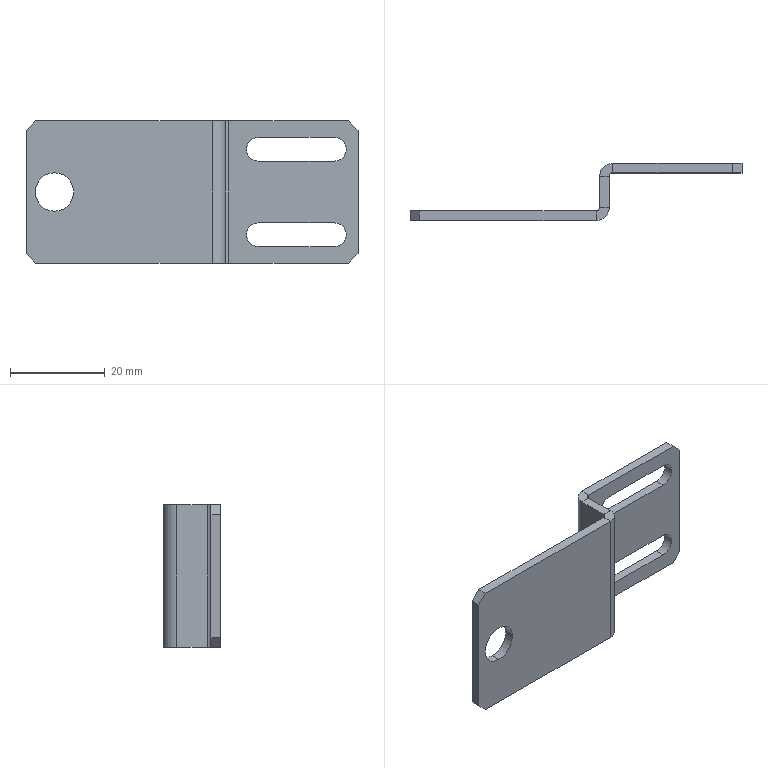Part | STEP file | 11-FG-SJ01111 | 1 solid | 36 faces | box 70 x 12 x 30 mm | volume 4193 mm3 | plane 26 | cylinder 10 | commonest cylinder face diameters 5 x4 1.473 x2 5.473 x2 8.1 x2
STEP:
#1=CARTESIAN_POINT('',(6.,0.,10.95));
#2=VERTEX_POINT('',#1);
#3=CARTESIAN_POINT('',(6.,0.,19.05));
#4=VERTEX_POINT('',#3);
#5=CARTESIAN_POINT('',(6.,0.,15.));
#6=DIRECTION('',(0.,1.,0.));
#7=DIRECTION('',(0.,0.,1.));
#8=AXIS2_PLACEMENT_3D('',#5,#6,#7);
#9=CIRCLE('',#8,4.05);
#10=EDGE_CURVE('',#2,#4,#9,.T.);
#11=ORIENTED_EDGE('',*,*,#10,.T.);
#12=CARTESIAN_POINT('',(6.,-2.,19.05));
#13=VERTEX_POINT('',#12);
#14=CARTESIAN_POINT('',(6.,8.,19.05));
#15=DIRECTION('',(0.,-1.,0.));
#16=VECTOR('',#15,1000.);
#17=LINE('',#14,#16);
#18=EDGE_CURVE('',#4,#13,#17,.T.);
#19=ORIENTED_EDGE('',*,*,#18,.T.);
#20=CARTESIAN_POINT('',(6.,-2.,10.95));
#21=VERTEX_POINT('',#20);
#22=CARTESIAN_POINT('',(6.,-2.,15.));
#23=DIRECTION('',(0.,-1.,0.));
#24=DIRECTION('',(0.,0.,-1.));
#25=AXIS2_PLACEMENT_3D('',#22,#23,#24);
#26=CIRCLE('',#25,4.05);
#27=EDGE_CURVE('',#13,#21,#26,.T.);
#28=ORIENTED_EDGE('',*,*,#27,.T.);
#29=CARTESIAN_POINT('',(6.,8.,10.95));
#30=DIRECTION('',(0.,-1.,0.));
#31=VECTOR('',#30,1000.);
#32=LINE('',#29,#31);
#33=EDGE_CURVE('',#2,#21,#32,.T.);
#34=ORIENTED_EDGE('',*,*,#33,.F.);
#35=EDGE_LOOP('',(#11,#19,#28,#34));
#36=FACE_OUTER_BOUND('',#35,.T.);
#37=CARTESIAN_POINT('',(6.,8.,15.));
#38=DIRECTION('',(0.,-1.,0.));
#39=DIRECTION('',(0.,0.,-1.));
#40=AXIS2_PLACEMENT_3D('',#37,#38,#39);
#41=CYLINDRICAL_SURFACE('',#40,4.05);
#42=ADVANCED_FACE('',(#36),#41,.F.);
#43=CARTESIAN_POINT('',(40.,0.7366,30.));
#44=VERTEX_POINT('',#43);
#45=CARTESIAN_POINT('',(42.,0.7366,30.));
#46=VERTEX_POINT('',#45);
#47=CARTESIAN_POINT('',(40.,0.7366,30.));
#48=DIRECTION('',(1.,0.,0.));
#49=VECTOR('',#48,1000.);
#50=LINE('',#47,#49);
#51=EDGE_CURVE('',#44,#46,#50,.T.);
#52=ORIENTED_EDGE('',*,*,#51,.F.);
#53=CARTESIAN_POINT('',(39.263,0.,30.));
#54=VERTEX_POINT('',#53);
#55=CARTESIAN_POINT('',(39.263,0.7366,30.));
#56=DIRECTION('',(0.,0.,1.));
#57=DIRECTION('',(-1.,0.,0.));
#58=AXIS2_PLACEMENT_3D('',#55,#56,#57);
#59=CIRCLE('',#58,0.7366);
#60=EDGE_CURVE('',#54,#44,#59,.T.);
#61=ORIENTED_EDGE('',*,*,#60,.F.);
#62=CARTESIAN_POINT('',(39.263,-2.,30.));
#63=VERTEX_POINT('',#62);
#64=CARTESIAN_POINT('',(39.263,-2.,30.));
#65=DIRECTION('',(0.,1.,0.));
#66=VECTOR('',#65,1000.);
#67=LINE('',#64,#66);
#68=EDGE_CURVE('',#63,#54,#67,.T.);
#69=ORIENTED_EDGE('',*,*,#68,.F.);
#70=CARTESIAN_POINT('',(39.263,0.7366,30.));
#71=DIRECTION('',(0.,0.,1.));
#72=DIRECTION('',(1.,0.,0.));
#73=AXIS2_PLACEMENT_3D('',#70,#71,#72);
#74=CIRCLE('',#73,2.737);
#75=EDGE_CURVE('',#63,#46,#74,.T.);
#76=ORIENTED_EDGE('',*,*,#75,.T.);
#77=EDGE_LOOP('',(#52,#61,#69,#76));
#78=FACE_OUTER_BOUND('',#77,.T.);
#79=CARTESIAN_POINT('',(40.,0.7366,30.));
#80=DIRECTION('',(0.,0.,1.));
#81=DIRECTION('',(1.,0.,0.));
#82=AXIS2_PLACEMENT_3D('',#79,#80,#81);
#83=PLANE('',#82);
#84=ADVANCED_FACE('',(#78),#83,.T.);
#85=CARTESIAN_POINT('',(40.,7.263,30.));
#86=VERTEX_POINT('',#85);
#87=CARTESIAN_POINT('',(40.,0.,30.));
#88=DIRECTION('',(0.,1.,0.));
#89=VECTOR('',#88,1000.);
#90=LINE('',#87,#89);
#91=EDGE_CURVE('',#44,#86,#90,.T.);
#92=ORIENTED_EDGE('',*,*,#91,.F.);
#93=ORIENTED_EDGE('',*,*,#51,.T.);
#94=CARTESIAN_POINT('',(42.,7.263,30.));
#95=VERTEX_POINT('',#94);
#96=CARTESIAN_POINT('',(42.,0.,30.));
#97=DIRECTION('',(0.,1.,0.));
#98=VECTOR('',#97,1000.);
#99=LINE('',#96,#98);
#100=EDGE_CURVE('',#46,#95,#99,.T.);
#101=ORIENTED_EDGE('',*,*,#100,.T.);
#102=CARTESIAN_POINT('',(42.,7.263,30.));
#103=DIRECTION('',(-1.,0.,0.));
#104=VECTOR('',#103,1000.);
#105=LINE('',#102,#104);
#106=EDGE_CURVE('',#95,#86,#105,.T.);
#107=ORIENTED_EDGE('',*,*,#106,.T.);
#108=EDGE_LOOP('',(#92,#93,#101,#107));
#109=FACE_OUTER_BOUND('',#108,.T.);
#110=CARTESIAN_POINT('',(39.263,-2.,30.));
#111=DIRECTION('',(0.,0.,1.));
#112=DIRECTION('',(1.,0.,0.));
#113=AXIS2_PLACEMENT_3D('',#110,#111,#112);
#114=PLANE('',#113);
#115=ADVANCED_FACE('',(#109),#114,.T.);
#116=CARTESIAN_POINT('',(39.263,0.,0.));
#117=VERTEX_POINT('',#116);
#118=CARTESIAN_POINT('',(39.263,-2.,0.));
#119=VERTEX_POINT('',#118);
#120=CARTESIAN_POINT('',(39.263,0.,0.));
#121=DIRECTION('',(0.,-1.,0.));
#122=VECTOR('',#121,1000.);
#123=LINE('',#120,#122);
#124=EDGE_CURVE('',#117,#119,#123,.T.);
#125=ORIENTED_EDGE('',*,*,#124,.F.);
#126=CARTESIAN_POINT('',(40.,0.7366,0.));
#127=VERTEX_POINT('',#126);
#128=CARTESIAN_POINT('',(39.263,0.7366,0.));
#129=DIRECTION('',(0.,0.,1.));
#130=DIRECTION('',(-1.,0.,0.));
#131=AXIS2_PLACEMENT_3D('',#128,#129,#130);
#132=CIRCLE('',#131,0.7366);
#133=EDGE_CURVE('',#117,#127,#132,.T.);
#134=ORIENTED_EDGE('',*,*,#133,.T.);
#135=CARTESIAN_POINT('',(42.,0.7366,0.));
#136=VERTEX_POINT('',#135);
#137=CARTESIAN_POINT('',(42.,0.7366,0.));
#138=DIRECTION('',(-1.,0.,0.));
#139=VECTOR('',#138,1000.);
#140=LINE('',#137,#139);
#141=EDGE_CURVE('',#136,#127,#140,.T.);
#142=ORIENTED_EDGE('',*,*,#141,.F.);
#143=CARTESIAN_POINT('',(39.263,0.7366,0.));
#144=DIRECTION('',(0.,0.,1.));
#145=DIRECTION('',(1.,0.,0.));
#146=AXIS2_PLACEMENT_3D('',#143,#144,#145);
#147=CIRCLE('',#146,2.737);
#148=EDGE_CURVE('',#119,#136,#147,.T.);
#149=ORIENTED_EDGE('',*,*,#148,.F.);
#150=EDGE_LOOP('',(#125,#134,#142,#149));
#151=FACE_OUTER_BOUND('',#150,.T.);
#152=CARTESIAN_POINT('',(39.263,0.,0.));
#153=DIRECTION('',(0.,0.,-1.));
#154=DIRECTION('',(-1.,0.,0.));
#155=AXIS2_PLACEMENT_3D('',#152,#153,#154);
#156=PLANE('',#155);
#157=ADVANCED_FACE('',(#151),#156,.T.);
#158=CARTESIAN_POINT('',(2.,-2.,0.));
#159=VERTEX_POINT('',#158);
#160=CARTESIAN_POINT('',(0.,-2.,0.));
#161=DIRECTION('',(1.,0.,0.));
#162=VECTOR('',#161,1000.);
#163=LINE('',#160,#162);
#164=EDGE_CURVE('',#159,#119,#163,.T.);
#165=ORIENTED_EDGE('',*,*,#164,.F.);
#166=CARTESIAN_POINT('',(2.,0.,0.));
#167=VERTEX_POINT('',#166);
#168=CARTESIAN_POINT('',(2.,0.7366,0.));
#169=DIRECTION('',(0.,1.,0.));
#170=VECTOR('',#169,1000.);
#171=LINE('',#168,#170);
#172=EDGE_CURVE('',#159,#167,#171,.T.);
#173=ORIENTED_EDGE('',*,*,#172,.T.);
#174=CARTESIAN_POINT('',(0.,0.,0.));
#175=DIRECTION('',(1.,0.,0.));
#176=VECTOR('',#175,1000.);
#177=LINE('',#174,#176);
#178=EDGE_CURVE('',#167,#117,#177,.T.);
#179=ORIENTED_EDGE('',*,*,#178,.T.);
#180=ORIENTED_EDGE('',*,*,#124,.T.);
#181=EDGE_LOOP('',(#165,#173,#179,#180));
#182=FACE_OUTER_BOUND('',#181,.T.);
#183=CARTESIAN_POINT('',(42.,0.7366,0.));
#184=DIRECTION('',(0.,0.,-1.));
#185=DIRECTION('',(-1.,0.,0.));
#186=AXIS2_PLACEMENT_3D('',#183,#184,#185);
#187=PLANE('',#186);
#188=ADVANCED_FACE('',(#182),#187,.T.);
#189=CARTESIAN_POINT('',(42.737,10.,30.));
#190=VERTEX_POINT('',#189);
#191=CARTESIAN_POINT('',(42.737,8.,30.));
#192=VERTEX_POINT('',#191);
#193=CARTESIAN_POINT('',(42.737,10.,30.));
#194=DIRECTION('',(0.,-1.,0.));
#195=VECTOR('',#194,1000.);
#196=LINE('',#193,#195);
#197=EDGE_CURVE('',#190,#192,#196,.T.);
#198=ORIENTED_EDGE('',*,*,#197,.F.);
#199=CARTESIAN_POINT('',(42.737,7.263,30.));
#200=DIRECTION('',(0.,0.,-1.));
#201=DIRECTION('',(1.,0.,0.));
#202=AXIS2_PLACEMENT_3D('',#199,#200,#201);
#203=CIRCLE('',#202,2.737);
#204=EDGE_CURVE('',#86,#190,#203,.T.);
#205=ORIENTED_EDGE('',*,*,#204,.F.);
#206=ORIENTED_EDGE('',*,*,#106,.F.);
#207=CARTESIAN_POINT('',(42.737,7.263,30.));
#208=DIRECTION('',(0.,0.,-1.));
#209=DIRECTION('',(1.,0.,0.));
#210=AXIS2_PLACEMENT_3D('',#207,#208,#209);
#211=CIRCLE('',#210,0.7366);
#212=EDGE_CURVE('',#95,#192,#211,.T.);
#213=ORIENTED_EDGE('',*,*,#212,.T.);
#214=EDGE_LOOP('',(#198,#205,#206,#213));
#215=FACE_OUTER_BOUND('',#214,.T.);
#216=CARTESIAN_POINT('',(42.737,10.,30.));
#217=DIRECTION('',(0.,0.,1.));
#218=DIRECTION('',(1.,0.,0.));
#219=AXIS2_PLACEMENT_3D('',#216,#217,#218);
#220=PLANE('',#219);
#221=ADVANCED_FACE('',(#215),#220,.T.);
#222=CARTESIAN_POINT('',(68.,8.,30.));
#223=VERTEX_POINT('',#222);
#224=CARTESIAN_POINT('',(40.,8.,30.));
#225=DIRECTION('',(1.,0.,0.));
#226=VECTOR('',#225,1000.);
#227=LINE('',#224,#226);
#228=EDGE_CURVE('',#192,#223,#227,.T.);
#229=ORIENTED_EDGE('',*,*,#228,.T.);
#230=CARTESIAN_POINT('',(68.,10.,30.));
#231=VERTEX_POINT('',#230);
#232=CARTESIAN_POINT('',(68.,7.263,30.));
#233=DIRECTION('',(0.,1.,0.));
#234=VECTOR('',#233,1000.);
#235=LINE('',#232,#234);
#236=EDGE_CURVE('',#223,#231,#235,.T.);
#237=ORIENTED_EDGE('',*,*,#236,.T.);
#238=CARTESIAN_POINT('',(40.,10.,30.));
#239=DIRECTION('',(1.,0.,0.));
#240=VECTOR('',#239,1000.);
#241=LINE('',#238,#240);
#242=EDGE_CURVE('',#190,#231,#241,.T.);
#243=ORIENTED_EDGE('',*,*,#242,.F.);
#244=ORIENTED_EDGE('',*,*,#197,.T.);
#245=EDGE_LOOP('',(#229,#237,#243,#244));
#246=FACE_OUTER_BOUND('',#245,.T.);
#247=CARTESIAN_POINT('',(42.,7.263,30.));
#248=DIRECTION('',(0.,0.,1.));
#249=DIRECTION('',(1.,0.,0.));
#250=AXIS2_PLACEMENT_3D('',#247,#248,#249);
#251=PLANE('',#250);
#252=ADVANCED_FACE('',(#246),#251,.T.);
#253=CARTESIAN_POINT('',(40.,7.263,0.));
#254=VERTEX_POINT('',#253);
#255=CARTESIAN_POINT('',(42.,7.263,0.));
#256=VERTEX_POINT('',#255);
#257=CARTESIAN_POINT('',(40.,7.263,0.));
#258=DIRECTION('',(1.,0.,0.));
#259=VECTOR('',#258,1000.);
#260=LINE('',#257,#259);
#261=EDGE_CURVE('',#254,#256,#260,.T.);
#262=ORIENTED_EDGE('',*,*,#261,.F.);
#263=CARTESIAN_POINT('',(42.737,10.,0.));
#264=VERTEX_POINT('',#263);
#265=CARTESIAN_POINT('',(42.737,7.263,0.));
#266=DIRECTION('',(0.,0.,-1.));
#267=DIRECTION('',(1.,0.,0.));
#268=AXIS2_PLACEMENT_3D('',#265,#266,#267);
#269=CIRCLE('',#268,2.737);
#270=EDGE_CURVE('',#254,#264,#269,.T.);
#271=ORIENTED_EDGE('',*,*,#270,.T.);
#272=CARTESIAN_POINT('',(42.737,8.,0.));
#273=VERTEX_POINT('',#272);
#274=CARTESIAN_POINT('',(42.737,8.,0.));
#275=DIRECTION('',(0.,1.,0.));
#276=VECTOR('',#275,1000.);
#277=LINE('',#274,#276);
#278=EDGE_CURVE('',#273,#264,#277,.T.);
#279=ORIENTED_EDGE('',*,*,#278,.F.);
#280=CARTESIAN_POINT('',(42.737,7.263,0.));
#281=DIRECTION('',(0.,0.,-1.));
#282=DIRECTION('',(1.,0.,0.));
#283=AXIS2_PLACEMENT_3D('',#280,#281,#282);
#284=CIRCLE('',#283,0.7366);
#285=EDGE_CURVE('',#256,#273,#284,.T.);
#286=ORIENTED_EDGE('',*,*,#285,.F.);
#287=EDGE_LOOP('',(#262,#271,#279,#286));
#288=FACE_OUTER_BOUND('',#287,.T.);
#289=CARTESIAN_POINT('',(40.,7.263,0.));
#290=DIRECTION('',(0.,0.,-1.));
#291=DIRECTION('',(-1.,0.,0.));
#292=AXIS2_PLACEMENT_3D('',#289,#290,#291);
#293=PLANE('',#292);
#294=ADVANCED_FACE('',(#288),#293,.T.);
#295=CARTESIAN_POINT('',(40.,0.,0.));
#296=DIRECTION('',(0.,1.,0.));
#297=VECTOR('',#296,1000.);
#298=LINE('',#295,#297);
#299=EDGE_CURVE('',#127,#254,#298,.T.);
#300=ORIENTED_EDGE('',*,*,#299,.T.);
#301=ORIENTED_EDGE('',*,*,#261,.T.);
#302=CARTESIAN_POINT('',(42.,0.,0.));
#303=DIRECTION('',(0.,1.,0.));
#304=VECTOR('',#303,1000.);
#305=LINE('',#302,#304);
#306=EDGE_CURVE('',#136,#256,#305,.T.);
#307=ORIENTED_EDGE('',*,*,#306,.F.);
#308=ORIENTED_EDGE('',*,*,#141,.T.);
#309=EDGE_LOOP('',(#300,#301,#307,#308));
#310=FACE_OUTER_BOUND('',#309,.T.);
#311=CARTESIAN_POINT('',(42.737,8.,0.));
#312=DIRECTION('',(0.,0.,-1.));
#313=DIRECTION('',(-1.,0.,0.));
#314=AXIS2_PLACEMENT_3D('',#311,#312,#313);
#315=PLANE('',#314);
#316=ADVANCED_FACE('',(#310),#315,.T.);
#317=CARTESIAN_POINT('',(65.,8.,21.5));
#318=VERTEX_POINT('',#317);
#319=CARTESIAN_POINT('',(49.,8.,21.5));
#320=VERTEX_POINT('',#319);
#321=CARTESIAN_POINT('',(40.,8.,21.5));
#322=DIRECTION('',(-1.,0.,0.));
#323=VECTOR('',#322,1000.);
#324=LINE('',#321,#323);
#325=EDGE_CURVE('',#318,#320,#324,.T.);
#326=ORIENTED_EDGE('',*,*,#325,.T.);
#327=CARTESIAN_POINT('',(49.,8.,26.5));
#328=VERTEX_POINT('',#327);
#329=CARTESIAN_POINT('',(49.,8.,24.));
#330=DIRECTION('',(0.,1.,0.));
#331=DIRECTION('',(0.,0.,1.));
#332=AXIS2_PLACEMENT_3D('',#329,#330,#331);
#333=CIRCLE('',#332,2.5);
#334=EDGE_CURVE('',#320,#328,#333,.T.);
#335=ORIENTED_EDGE('',*,*,#334,.T.);
#336=CARTESIAN_POINT('',(65.,8.,26.5));
#337=VERTEX_POINT('',#336);
#338=CARTESIAN_POINT('',(40.,8.,26.5));
#339=DIRECTION('',(1.,0.,0.));
#340=VECTOR('',#339,1000.);
#341=LINE('',#338,#340);
#342=EDGE_CURVE('',#328,#337,#341,.T.);
#343=ORIENTED_EDGE('',*,*,#342,.T.);
#344=CARTESIAN_POINT('',(65.,8.,24.));
#345=DIRECTION('',(0.,1.,0.));
#346=DIRECTION('',(0.,0.,1.));
#347=AXIS2_PLACEMENT_3D('',#344,#345,#346);
#348=CIRCLE('',#347,2.5);
#349=EDGE_CURVE('',#337,#318,#348,.T.);
#350=ORIENTED_EDGE('',*,*,#349,.T.);
#351=EDGE_LOOP('',(#326,#335,#343,#350));
#352=FACE_BOUND('',#351,.T.);
#353=CARTESIAN_POINT('',(65.,8.,3.5));
#354=VERTEX_POINT('',#353);
#355=CARTESIAN_POINT('',(49.,8.,3.5));
#356=VERTEX_POINT('',#355);
#357=CARTESIAN_POINT('',(40.,8.,3.5));
#358=DIRECTION('',(-1.,0.,0.));
#359=VECTOR('',#358,1000.);
#360=LINE('',#357,#359);
#361=EDGE_CURVE('',#354,#356,#360,.T.);
#362=ORIENTED_EDGE('',*,*,#361,.T.);
#363=CARTESIAN_POINT('',(49.,8.,8.5));
#364=VERTEX_POINT('',#363);
#365=CARTESIAN_POINT('',(49.,8.,6.));
#366=DIRECTION('',(0.,1.,0.));
#367=DIRECTION('',(0.,0.,1.));
#368=AXIS2_PLACEMENT_3D('',#365,#366,#367);
#369=CIRCLE('',#368,2.5);
#370=EDGE_CURVE('',#356,#364,#369,.T.);
#371=ORIENTED_EDGE('',*,*,#370,.T.);
#372=CARTESIAN_POINT('',(65.,8.,8.5));
#373=VERTEX_POINT('',#372);
#374=CARTESIAN_POINT('',(40.,8.,8.5));
#375=DIRECTION('',(1.,0.,0.));
#376=VECTOR('',#375,1000.);
#377=LINE('',#374,#376);
#378=EDGE_CURVE('',#364,#373,#377,.T.);
#379=ORIENTED_EDGE('',*,*,#378,.T.);
#380=CARTESIAN_POINT('',(65.,8.,6.));
#381=DIRECTION('',(0.,1.,0.));
#382=DIRECTION('',(0.,0.,1.));
#383=AXIS2_PLACEMENT_3D('',#380,#381,#382);
#384=CIRCLE('',#383,2.5);
#385=EDGE_CURVE('',#373,#354,#384,.T.);
#386=ORIENTED_EDGE('',*,*,#385,.T.);
#387=EDGE_LOOP('',(#362,#371,#379,#386));
#388=FACE_BOUND('',#387,.T.);
#389=CARTESIAN_POINT('',(68.,8.,0.));
#390=VERTEX_POINT('',#389);
#391=CARTESIAN_POINT('',(40.,8.,0.));
#392=DIRECTION('',(1.,0.,0.));
#393=VECTOR('',#392,1000.);
#394=LINE('',#391,#393);
#395=EDGE_CURVE('',#273,#390,#394,.T.);
#396=ORIENTED_EDGE('',*,*,#395,.T.);
#397=CARTESIAN_POINT('',(70.,8.,2.));
#398=VERTEX_POINT('',#397);
#399=CARTESIAN_POINT('',(68.,8.,0.));
#400=DIRECTION('',(0.7071,0.,0.7071));
#401=VECTOR('',#400,1000.);
#402=LINE('',#399,#401);
#403=EDGE_CURVE('',#390,#398,#402,.T.);
#404=ORIENTED_EDGE('',*,*,#403,.T.);
#405=CARTESIAN_POINT('',(70.,8.,28.));
#406=VERTEX_POINT('',#405);
#407=CARTESIAN_POINT('',(70.,8.,30.));
#408=DIRECTION('',(0.,0.,-1.));
#409=VECTOR('',#408,1000.);
#410=LINE('',#407,#409);
#411=EDGE_CURVE('',#406,#398,#410,.T.);
#412=ORIENTED_EDGE('',*,*,#411,.F.);
#413=CARTESIAN_POINT('',(70.,8.,28.));
#414=DIRECTION('',(-0.7071,0.,0.7071));
#415=VECTOR('',#414,1000.);
#416=LINE('',#413,#415);
#417=EDGE_CURVE('',#406,#223,#416,.T.);
#418=ORIENTED_EDGE('',*,*,#417,.T.);
#419=ORIENTED_EDGE('',*,*,#228,.F.);
#420=CARTESIAN_POINT('',(42.737,8.,30.));
#421=DIRECTION('',(0.,0.,-1.));
#422=VECTOR('',#421,1000.);
#423=LINE('',#420,#422);
#424=EDGE_CURVE('',#192,#273,#423,.T.);
#425=ORIENTED_EDGE('',*,*,#424,.T.);
#426=EDGE_LOOP('',(#396,#404,#412,#418,#419,#425));
#427=FACE_OUTER_BOUND('',#426,.T.);
#428=CARTESIAN_POINT('',(40.,8.,30.));
#429=DIRECTION('',(0.,1.,0.));
#430=DIRECTION('',(0.,0.,1.));
#431=AXIS2_PLACEMENT_3D('',#428,#429,#430);
#432=PLANE('',#431);
#433=ADVANCED_FACE('',(#352,#388,#427),#432,.F.);
#434=ORIENTED_EDGE('',*,*,#411,.T.);
#435=CARTESIAN_POINT('',(70.,10.,2.));
#436=VERTEX_POINT('',#435);
#437=CARTESIAN_POINT('',(70.,10.,2.));
#438=DIRECTION('',(0.,1.,0.));
#439=VECTOR('',#438,1000.);
#440=LINE('',#437,#439);
#441=EDGE_CURVE('',#398,#436,#440,.T.);
#442=ORIENTED_EDGE('',*,*,#441,.T.);
#443=CARTESIAN_POINT('',(70.,10.,28.));
#444=VERTEX_POINT('',#443);
#445=CARTESIAN_POINT('',(70.,10.,30.));
#446=DIRECTION('',(0.,0.,-1.));
#447=VECTOR('',#446,1000.);
#448=LINE('',#445,#447);
#449=EDGE_CURVE('',#444,#436,#448,.T.);
#450=ORIENTED_EDGE('',*,*,#449,.F.);
#451=CARTESIAN_POINT('',(70.,10.,28.));
#452=DIRECTION('',(0.,-1.,0.));
#453=VECTOR('',#452,1000.);
#454=LINE('',#451,#453);
#455=EDGE_CURVE('',#444,#406,#454,.T.);
#456=ORIENTED_EDGE('',*,*,#455,.T.);
#457=EDGE_LOOP('',(#434,#442,#450,#456));
#458=FACE_OUTER_BOUND('',#457,.T.);
#459=CARTESIAN_POINT('',(70.,10.,30.));
#460=DIRECTION('',(1.,0.,0.));
#461=DIRECTION('',(0.,0.,-1.));
#462=AXIS2_PLACEMENT_3D('',#459,#460,#461);
#463=PLANE('',#462);
#464=ADVANCED_FACE('',(#458),#463,.T.);
#465=CARTESIAN_POINT('',(49.,10.,21.5));
#466=VERTEX_POINT('',#465);
#467=CARTESIAN_POINT('',(49.,10.,26.5));
#468=VERTEX_POINT('',#467);
#469=CARTESIAN_POINT('',(49.,10.,24.));
#470=DIRECTION('',(0.,1.,0.));
#471=DIRECTION('',(0.,0.,-1.));
#472=AXIS2_PLACEMENT_3D('',#469,#470,#471);
#473=CIRCLE('',#472,2.5);
#474=EDGE_CURVE('',#466,#468,#473,.T.);
#475=ORIENTED_EDGE('',*,*,#474,.F.);
#476=CARTESIAN_POINT('',(65.,10.,21.5));
#477=VERTEX_POINT('',#476);
#478=CARTESIAN_POINT('',(49.,10.,21.5));
#479=DIRECTION('',(-1.,0.,0.));
#480=VECTOR('',#479,1000.);
#481=LINE('',#478,#480);
#482=EDGE_CURVE('',#477,#466,#481,.T.);
#483=ORIENTED_EDGE('',*,*,#482,.F.);
#484=CARTESIAN_POINT('',(65.,10.,26.5));
#485=VERTEX_POINT('',#484);
#486=CARTESIAN_POINT('',(65.,10.,24.));
#487=DIRECTION('',(0.,1.,0.));
#488=DIRECTION('',(0.,0.,-1.));
#489=AXIS2_PLACEMENT_3D('',#486,#487,#488);
#490=CIRCLE('',#489,2.5);
#491=EDGE_CURVE('',#485,#477,#490,.T.);
#492=ORIENTED_EDGE('',*,*,#491,.F.);
#493=CARTESIAN_POINT('',(49.,10.,26.5));
#494=DIRECTION('',(1.,0.,0.));
#495=VECTOR('',#494,1000.);
#496=LINE('',#493,#495);
#497=EDGE_CURVE('',#468,#485,#496,.T.);
#498=ORIENTED_EDGE('',*,*,#497,.F.);
#499=EDGE_LOOP('',(#475,#483,#492,#498));
#500=FACE_BOUND('',#499,.T.);
#501=CARTESIAN_POINT('',(49.,10.,3.5));
#502=VERTEX_POINT('',#501);
#503=CARTESIAN_POINT('',(49.,10.,8.5));
#504=VERTEX_POINT('',#503);
#505=CARTESIAN_POINT('',(49.,10.,6.));
#506=DIRECTION('',(0.,1.,0.));
#507=DIRECTION('',(0.,0.,1.));
#508=AXIS2_PLACEMENT_3D('',#505,#506,#507);
#509=CIRCLE('',#508,2.5);
#510=EDGE_CURVE('',#502,#504,#509,.T.);
#511=ORIENTED_EDGE('',*,*,#510,.F.);
#512=CARTESIAN_POINT('',(65.,10.,3.5));
#513=VERTEX_POINT('',#512);
#514=CARTESIAN_POINT('',(49.,10.,3.5));
#515=DIRECTION('',(-1.,0.,0.));
#516=VECTOR('',#515,1000.);
#517=LINE('',#514,#516);
#518=EDGE_CURVE('',#513,#502,#517,.T.);
#519=ORIENTED_EDGE('',*,*,#518,.F.);
#520=CARTESIAN_POINT('',(65.,10.,8.5));
#521=VERTEX_POINT('',#520);
#522=CARTESIAN_POINT('',(65.,10.,6.));
#523=DIRECTION('',(0.,1.,0.));
#524=DIRECTION('',(0.,0.,1.));
#525=AXIS2_PLACEMENT_3D('',#522,#523,#524);
#526=CIRCLE('',#525,2.5);
#527=EDGE_CURVE('',#521,#513,#526,.T.);
#528=ORIENTED_EDGE('',*,*,#527,.F.);
#529=CARTESIAN_POINT('',(49.,10.,8.5));
#530=DIRECTION('',(1.,0.,0.));
#531=VECTOR('',#530,1000.);
#532=LINE('',#529,#531);
#533=EDGE_CURVE('',#504,#521,#532,.T.);
#534=ORIENTED_EDGE('',*,*,#533,.F.);
#535=EDGE_LOOP('',(#511,#519,#528,#534));
#536=FACE_BOUND('',#535,.T.);
#537=ORIENTED_EDGE('',*,*,#449,.T.);
#538=CARTESIAN_POINT('',(68.,10.,0.));
#539=VERTEX_POINT('',#538);
#540=CARTESIAN_POINT('',(69.,10.,1.));
#541=DIRECTION('',(-0.7071,0.,-0.7071));
#542=VECTOR('',#541,1000.);
#543=LINE('',#540,#542);
#544=EDGE_CURVE('',#436,#539,#543,.T.);
#545=ORIENTED_EDGE('',*,*,#544,.T.);
#546=CARTESIAN_POINT('',(40.,10.,0.));
#547=DIRECTION('',(1.,0.,0.));
#548=VECTOR('',#547,1000.);
#549=LINE('',#546,#548);
#550=EDGE_CURVE('',#264,#539,#549,.T.);
#551=ORIENTED_EDGE('',*,*,#550,.F.);
#552=CARTESIAN_POINT('',(42.737,10.,30.));
#553=DIRECTION('',(0.,0.,-1.));
#554=VECTOR('',#553,1000.);
#555=LINE('',#552,#554);
#556=EDGE_CURVE('',#190,#264,#555,.T.);
#557=ORIENTED_EDGE('',*,*,#556,.F.);
#558=ORIENTED_EDGE('',*,*,#242,.T.);
#559=CARTESIAN_POINT('',(54.,10.,44.));
#560=DIRECTION('',(0.7071,0.,-0.7071));
#561=VECTOR('',#560,1000.);
#562=LINE('',#559,#561);
#563=EDGE_CURVE('',#231,#444,#562,.T.);
#564=ORIENTED_EDGE('',*,*,#563,.T.);
#565=EDGE_LOOP('',(#537,#545,#551,#557,#558,#564));
#566=FACE_OUTER_BOUND('',#565,.T.);
#567=CARTESIAN_POINT('',(40.,10.,30.));
#568=DIRECTION('',(0.,1.,0.));
#569=DIRECTION('',(0.,0.,1.));
#570=AXIS2_PLACEMENT_3D('',#567,#568,#569);
#571=PLANE('',#570);
#572=ADVANCED_FACE('',(#500,#536,#566),#571,.T.);
#573=ORIENTED_EDGE('',*,*,#270,.F.);
#574=CARTESIAN_POINT('',(40.,7.263,30.));
#575=DIRECTION('',(0.,0.,-1.));
#576=VECTOR('',#575,1000.);
#577=LINE('',#574,#576);
#578=EDGE_CURVE('',#86,#254,#577,.T.);
#579=ORIENTED_EDGE('',*,*,#578,.F.);
#580=ORIENTED_EDGE('',*,*,#204,.T.);
#581=ORIENTED_EDGE('',*,*,#556,.T.);
#582=EDGE_LOOP('',(#573,#579,#580,#581));
#583=FACE_OUTER_BOUND('',#582,.T.);
#584=CARTESIAN_POINT('',(42.737,7.263,30.));
#585=DIRECTION('',(0.,0.,-1.));
#586=DIRECTION('',(-1.,0.,0.));
#587=AXIS2_PLACEMENT_3D('',#584,#585,#586);
#588=CYLINDRICAL_SURFACE('',#587,2.737);
#589=ADVANCED_FACE('',(#583),#588,.T.);
#590=ORIENTED_EDGE('',*,*,#299,.F.);
#591=CARTESIAN_POINT('',(40.,0.7366,30.));
#592=DIRECTION('',(0.,0.,-1.));
#593=VECTOR('',#592,1000.);
#594=LINE('',#591,#593);
#595=EDGE_CURVE('',#44,#127,#594,.T.);
#596=ORIENTED_EDGE('',*,*,#595,.F.);
#597=ORIENTED_EDGE('',*,*,#91,.T.);
#598=ORIENTED_EDGE('',*,*,#578,.T.);
#599=EDGE_LOOP('',(#590,#596,#597,#598));
#600=FACE_OUTER_BOUND('',#599,.T.);
#601=CARTESIAN_POINT('',(40.,0.,30.));
#602=DIRECTION('',(-1.,0.,0.));
#603=DIRECTION('',(0.,0.,1.));
#604=AXIS2_PLACEMENT_3D('',#601,#602,#603);
#605=PLANE('',#604);
#606=ADVANCED_FACE('',(#600),#605,.T.);
#607=ORIENTED_EDGE('',*,*,#133,.F.);
#608=CARTESIAN_POINT('',(39.263,0.,30.));
#609=DIRECTION('',(0.,0.,-1.));
#610=VECTOR('',#609,1000.);
#611=LINE('',#608,#610);
#612=EDGE_CURVE('',#54,#117,#611,.T.);
#613=ORIENTED_EDGE('',*,*,#612,.F.);
#614=ORIENTED_EDGE('',*,*,#60,.T.);
#615=ORIENTED_EDGE('',*,*,#595,.T.);
#616=EDGE_LOOP('',(#607,#613,#614,#615));
#617=FACE_OUTER_BOUND('',#616,.T.);
#618=CARTESIAN_POINT('',(39.263,0.7366,30.));
#619=DIRECTION('',(0.,0.,-1.));
#620=DIRECTION('',(-1.,0.,0.));
#621=AXIS2_PLACEMENT_3D('',#618,#619,#620);
#622=CYLINDRICAL_SURFACE('',#621,0.7366);
#623=ADVANCED_FACE('',(#617),#622,.F.);
#624=ORIENTED_EDGE('',*,*,#10,.F.);
#625=CARTESIAN_POINT('',(6.,0.,15.));
#626=DIRECTION('',(0.,1.,0.));
#627=DIRECTION('',(0.,0.,1.));
#628=AXIS2_PLACEMENT_3D('',#625,#626,#627);
#629=CIRCLE('',#628,4.05);
#630=EDGE_CURVE('',#4,#2,#629,.T.);
#631=ORIENTED_EDGE('',*,*,#630,.F.);
#632=EDGE_LOOP('',(#624,#631));
#633=FACE_BOUND('',#632,.T.);
#634=ORIENTED_EDGE('',*,*,#178,.F.);
#635=CARTESIAN_POINT('',(0.,0.,2.));
#636=VERTEX_POINT('',#635);
#637=CARTESIAN_POINT('',(-14.,0.,16.));
#638=DIRECTION('',(-0.7071,0.,0.7071));
#639=VECTOR('',#638,1000.);
#640=LINE('',#637,#639);
#641=EDGE_CURVE('',#167,#636,#640,.T.);
#642=ORIENTED_EDGE('',*,*,#641,.T.);
#643=CARTESIAN_POINT('',(0.,0.,28.));
#644=VERTEX_POINT('',#643);
#645=CARTESIAN_POINT('',(0.,0.,30.));
#646=DIRECTION('',(0.,0.,-1.));
#647=VECTOR('',#646,1000.);
#648=LINE('',#645,#647);
#649=EDGE_CURVE('',#644,#636,#648,.T.);
#650=ORIENTED_EDGE('',*,*,#649,.F.);
#651=CARTESIAN_POINT('',(2.,0.,30.));
#652=VERTEX_POINT('',#651);
#653=CARTESIAN_POINT('',(1.,0.,29.));
#654=DIRECTION('',(0.7071,0.,0.7071));
#655=VECTOR('',#654,1000.);
#656=LINE('',#653,#655);
#657=EDGE_CURVE('',#644,#652,#656,.T.);
#658=ORIENTED_EDGE('',*,*,#657,.T.);
#659=CARTESIAN_POINT('',(0.,0.,30.));
#660=DIRECTION('',(1.,0.,0.));
#661=VECTOR('',#660,1000.);
#662=LINE('',#659,#661);
#663=EDGE_CURVE('',#652,#54,#662,.T.);
#664=ORIENTED_EDGE('',*,*,#663,.T.);
#665=ORIENTED_EDGE('',*,*,#612,.T.);
#666=EDGE_LOOP('',(#634,#642,#650,#658,#664,#665));
#667=FACE_OUTER_BOUND('',#666,.T.);
#668=CARTESIAN_POINT('',(0.,0.,30.));
#669=DIRECTION('',(0.,1.,0.));
#670=DIRECTION('',(0.,0.,1.));
#671=AXIS2_PLACEMENT_3D('',#668,#669,#670);
#672=PLANE('',#671);
#673=ADVANCED_FACE('',(#633,#667),#672,.T.);
#674=ORIENTED_EDGE('',*,*,#649,.T.);
#675=CARTESIAN_POINT('',(0.,-2.,2.));
#676=VERTEX_POINT('',#675);
#677=CARTESIAN_POINT('',(0.,-2.,2.));
#678=DIRECTION('',(0.,-1.,0.));
#679=VECTOR('',#678,1000.);
#680=LINE('',#677,#679);
#681=EDGE_CURVE('',#636,#676,#680,.T.);
#682=ORIENTED_EDGE('',*,*,#681,.T.);
#683=CARTESIAN_POINT('',(0.,-2.,28.));
#684=VERTEX_POINT('',#683);
#685=CARTESIAN_POINT('',(0.,-2.,30.));
#686=DIRECTION('',(0.,0.,-1.));
#687=VECTOR('',#686,1000.);
#688=LINE('',#685,#687);
#689=EDGE_CURVE('',#684,#676,#688,.T.);
#690=ORIENTED_EDGE('',*,*,#689,.F.);
#691=CARTESIAN_POINT('',(0.,-2.,28.));
#692=DIRECTION('',(0.,1.,0.));
#693=VECTOR('',#692,1000.);
#694=LINE('',#691,#693);
#695=EDGE_CURVE('',#684,#644,#694,.T.);
#696=ORIENTED_EDGE('',*,*,#695,.T.);
#697=EDGE_LOOP('',(#674,#682,#690,#696));
#698=FACE_OUTER_BOUND('',#697,.T.);
#699=CARTESIAN_POINT('',(0.,-2.,30.));
#700=DIRECTION('',(-1.,0.,0.));
#701=DIRECTION('',(0.,0.,1.));
#702=AXIS2_PLACEMENT_3D('',#699,#700,#701);
#703=PLANE('',#702);
#704=ADVANCED_FACE('',(#698),#703,.T.);
#705=CARTESIAN_POINT('',(6.,-2.,15.));
#706=DIRECTION('',(0.,-1.,0.));
#707=DIRECTION('',(0.,0.,-1.));
#708=AXIS2_PLACEMENT_3D('',#705,#706,#707);
#709=CIRCLE('',#708,4.05);
#710=EDGE_CURVE('',#21,#13,#709,.T.);
#711=ORIENTED_EDGE('',*,*,#710,.F.);
#712=ORIENTED_EDGE('',*,*,#27,.F.);
#713=EDGE_LOOP('',(#711,#712));
#714=FACE_BOUND('',#713,.T.);
#715=ORIENTED_EDGE('',*,*,#689,.T.);
#716=CARTESIAN_POINT('',(2.,-2.,0.));
#717=DIRECTION('',(0.7071,0.,-0.7071));
#718=VECTOR('',#717,1000.);
#719=LINE('',#716,#718);
#720=EDGE_CURVE('',#676,#159,#719,.T.);
#721=ORIENTED_EDGE('',*,*,#720,.T.);
#722=ORIENTED_EDGE('',*,*,#164,.T.);
#723=CARTESIAN_POINT('',(39.263,-2.,30.));
#724=DIRECTION('',(0.,0.,-1.));
#725=VECTOR('',#724,1000.);
#726=LINE('',#723,#725);
#727=EDGE_CURVE('',#63,#119,#726,.T.);
#728=ORIENTED_EDGE('',*,*,#727,.F.);
#729=CARTESIAN_POINT('',(2.,-2.,30.));
#730=VERTEX_POINT('',#729);
#731=CARTESIAN_POINT('',(0.,-2.,30.));
#732=DIRECTION('',(1.,0.,0.));
#733=VECTOR('',#732,1000.);
#734=LINE('',#731,#733);
#735=EDGE_CURVE('',#730,#63,#734,.T.);
#736=ORIENTED_EDGE('',*,*,#735,.F.);
#737=CARTESIAN_POINT('',(0.,-2.,28.));
#738=DIRECTION('',(-0.7071,0.,-0.7071));
#739=VECTOR('',#738,1000.);
#740=LINE('',#737,#739);
#741=EDGE_CURVE('',#730,#684,#740,.T.);
#742=ORIENTED_EDGE('',*,*,#741,.T.);
#743=EDGE_LOOP('',(#715,#721,#722,#728,#736,#742));
#744=FACE_OUTER_BOUND('',#743,.T.);
#745=CARTESIAN_POINT('',(0.,-2.,30.));
#746=DIRECTION('',(0.,1.,0.));
#747=DIRECTION('',(0.,0.,1.));
#748=AXIS2_PLACEMENT_3D('',#745,#746,#747);
#749=PLANE('',#748);
#750=ADVANCED_FACE('',(#714,#744),#749,.F.);
#751=ORIENTED_EDGE('',*,*,#148,.T.);
#752=CARTESIAN_POINT('',(42.,0.7366,30.));
#753=DIRECTION('',(0.,0.,-1.));
#754=VECTOR('',#753,1000.);
#755=LINE('',#752,#754);
#756=EDGE_CURVE('',#46,#136,#755,.T.);
#757=ORIENTED_EDGE('',*,*,#756,.F.);
#758=ORIENTED_EDGE('',*,*,#75,.F.);
#759=ORIENTED_EDGE('',*,*,#727,.T.);
#760=EDGE_LOOP('',(#751,#757,#758,#759));
#761=FACE_OUTER_BOUND('',#760,.T.);
#762=CARTESIAN_POINT('',(39.263,0.7366,30.));
#763=DIRECTION('',(0.,0.,-1.));
#764=DIRECTION('',(-1.,0.,0.));
#765=AXIS2_PLACEMENT_3D('',#762,#763,#764);
#766=CYLINDRICAL_SURFACE('',#765,2.737);
#767=ADVANCED_FACE('',(#761),#766,.T.);
#768=ORIENTED_EDGE('',*,*,#306,.T.);
#769=CARTESIAN_POINT('',(42.,7.263,30.));
#770=DIRECTION('',(0.,0.,-1.));
#771=VECTOR('',#770,1000.);
#772=LINE('',#769,#771);
#773=EDGE_CURVE('',#95,#256,#772,.T.);
#774=ORIENTED_EDGE('',*,*,#773,.F.);
#775=ORIENTED_EDGE('',*,*,#100,.F.);
#776=ORIENTED_EDGE('',*,*,#756,.T.);
#777=EDGE_LOOP('',(#768,#774,#775,#776));
#778=FACE_OUTER_BOUND('',#777,.T.);
#779=CARTESIAN_POINT('',(42.,0.,30.));
#780=DIRECTION('',(-1.,0.,0.));
#781=DIRECTION('',(0.,0.,1.));
#782=AXIS2_PLACEMENT_3D('',#779,#780,#781);
#783=PLANE('',#782);
#784=ADVANCED_FACE('',(#778),#783,.F.);
#785=ORIENTED_EDGE('',*,*,#285,.T.);
#786=ORIENTED_EDGE('',*,*,#424,.F.);
#787=ORIENTED_EDGE('',*,*,#212,.F.);
#788=ORIENTED_EDGE('',*,*,#773,.T.);
#789=EDGE_LOOP('',(#785,#786,#787,#788));
#790=FACE_OUTER_BOUND('',#789,.T.);
#791=CARTESIAN_POINT('',(42.737,7.263,30.));
#792=DIRECTION('',(0.,0.,-1.));
#793=DIRECTION('',(-1.,0.,0.));
#794=AXIS2_PLACEMENT_3D('',#791,#792,#793);
#795=CYLINDRICAL_SURFACE('',#794,0.7366);
#796=ADVANCED_FACE('',(#790),#795,.F.);
#797=ORIENTED_EDGE('',*,*,#663,.F.);
#798=CARTESIAN_POINT('',(2.,7.263,30.));
#799=DIRECTION('',(0.,-1.,0.));
#800=VECTOR('',#799,1000.);
#801=LINE('',#798,#800);
#802=EDGE_CURVE('',#652,#730,#801,.T.);
#803=ORIENTED_EDGE('',*,*,#802,.T.);
#804=ORIENTED_EDGE('',*,*,#735,.T.);
#805=ORIENTED_EDGE('',*,*,#68,.T.);
#806=EDGE_LOOP('',(#797,#803,#804,#805));
#807=FACE_OUTER_BOUND('',#806,.T.);
#808=CARTESIAN_POINT('',(42.737,7.263,30.));
#809=DIRECTION('',(0.,0.,1.));
#810=DIRECTION('',(1.,0.,0.));
#811=AXIS2_PLACEMENT_3D('',#808,#809,#810);
#812=PLANE('',#811);
#813=ADVANCED_FACE('',(#807),#812,.T.);
#814=ORIENTED_EDGE('',*,*,#550,.T.);
#815=CARTESIAN_POINT('',(68.,8.,0.));
#816=DIRECTION('',(0.,-1.,0.));
#817=VECTOR('',#816,1000.);
#818=LINE('',#815,#817);
#819=EDGE_CURVE('',#539,#390,#818,.T.);
#820=ORIENTED_EDGE('',*,*,#819,.T.);
#821=ORIENTED_EDGE('',*,*,#395,.F.);
#822=ORIENTED_EDGE('',*,*,#278,.T.);
#823=EDGE_LOOP('',(#814,#820,#821,#822));
#824=FACE_OUTER_BOUND('',#823,.T.);
#825=CARTESIAN_POINT('',(42.737,7.263,0.));
#826=DIRECTION('',(0.,0.,1.));
#827=DIRECTION('',(1.,0.,0.));
#828=AXIS2_PLACEMENT_3D('',#825,#826,#827);
#829=PLANE('',#828);
#830=ADVANCED_FACE('',(#824),#829,.F.);
#831=ORIENTED_EDGE('',*,*,#18,.F.);
#832=ORIENTED_EDGE('',*,*,#630,.T.);
#833=ORIENTED_EDGE('',*,*,#33,.T.);
#834=ORIENTED_EDGE('',*,*,#710,.T.);
#835=EDGE_LOOP('',(#831,#832,#833,#834));
#836=FACE_OUTER_BOUND('',#835,.T.);
#837=CARTESIAN_POINT('',(6.,8.,15.));
#838=DIRECTION('',(0.,-1.,0.));
#839=DIRECTION('',(0.,0.,-1.));
#840=AXIS2_PLACEMENT_3D('',#837,#838,#839);
#841=CYLINDRICAL_SURFACE('',#840,4.05);
#842=ADVANCED_FACE('',(#836),#841,.F.);
#843=ORIENTED_EDGE('',*,*,#720,.F.);
#844=ORIENTED_EDGE('',*,*,#681,.F.);
#845=ORIENTED_EDGE('',*,*,#641,.F.);
#846=ORIENTED_EDGE('',*,*,#172,.F.);
#847=EDGE_LOOP('',(#843,#844,#845,#846));
#848=FACE_OUTER_BOUND('',#847,.T.);
#849=CARTESIAN_POINT('',(2.,0.7366,0.));
#850=DIRECTION('',(0.7071,0.,0.7071));
#851=DIRECTION('',(0.,1.,0.));
#852=AXIS2_PLACEMENT_3D('',#849,#850,#851);
#853=PLANE('',#852);
#854=ADVANCED_FACE('',(#848),#853,.F.);
#855=ORIENTED_EDGE('',*,*,#741,.F.);
#856=ORIENTED_EDGE('',*,*,#802,.F.);
#857=ORIENTED_EDGE('',*,*,#657,.F.);
#858=ORIENTED_EDGE('',*,*,#695,.F.);
#859=EDGE_LOOP('',(#855,#856,#857,#858));
#860=FACE_OUTER_BOUND('',#859,.T.);
#861=CARTESIAN_POINT('',(0.,-2.,28.));
#862=DIRECTION('',(0.7071,0.,-0.7071));
#863=DIRECTION('',(0.,1.,0.));
#864=AXIS2_PLACEMENT_3D('',#861,#862,#863);
#865=PLANE('',#864);
#866=ADVANCED_FACE('',(#860),#865,.F.);
#867=ORIENTED_EDGE('',*,*,#544,.F.);
#868=ORIENTED_EDGE('',*,*,#441,.F.);
#869=ORIENTED_EDGE('',*,*,#403,.F.);
#870=ORIENTED_EDGE('',*,*,#819,.F.);
#871=EDGE_LOOP('',(#867,#868,#869,#870));
#872=FACE_OUTER_BOUND('',#871,.T.);
#873=CARTESIAN_POINT('',(68.,7.263,0.));
#874=DIRECTION('',(0.7071,0.,-0.7071));
#875=DIRECTION('',(0.,1.,0.));
#876=AXIS2_PLACEMENT_3D('',#873,#874,#875);
#877=PLANE('',#876);
#878=ADVANCED_FACE('',(#872),#877,.T.);
#879=ORIENTED_EDGE('',*,*,#563,.F.);
#880=ORIENTED_EDGE('',*,*,#236,.F.);
#881=ORIENTED_EDGE('',*,*,#417,.F.);
#882=ORIENTED_EDGE('',*,*,#455,.F.);
#883=EDGE_LOOP('',(#879,#880,#881,#882));
#884=FACE_OUTER_BOUND('',#883,.T.);
#885=CARTESIAN_POINT('',(70.,10.,28.));
#886=DIRECTION('',(-0.7071,0.,-0.7071));
#887=DIRECTION('',(0.,-1.,0.));
#888=AXIS2_PLACEMENT_3D('',#885,#886,#887);
#889=PLANE('',#888);
#890=ADVANCED_FACE('',(#884),#889,.F.);
#891=CARTESIAN_POINT('',(49.,-2.,3.5));
#892=DIRECTION('',(0.,1.,0.));
#893=VECTOR('',#892,1000.);
#894=LINE('',#891,#893);
#895=EDGE_CURVE('',#356,#502,#894,.T.);
#896=ORIENTED_EDGE('',*,*,#895,.T.);
#897=ORIENTED_EDGE('',*,*,#510,.T.);
#898=CARTESIAN_POINT('',(49.,-2.,8.5));
#899=DIRECTION('',(0.,1.,0.));
#900=VECTOR('',#899,1000.);
#901=LINE('',#898,#900);
#902=EDGE_CURVE('',#364,#504,#901,.T.);
#903=ORIENTED_EDGE('',*,*,#902,.F.);
#904=ORIENTED_EDGE('',*,*,#370,.F.);
#905=EDGE_LOOP('',(#896,#897,#903,#904));
#906=FACE_OUTER_BOUND('',#905,.T.);
#907=CARTESIAN_POINT('',(49.,-2.,6.));
#908=DIRECTION('',(0.,1.,0.));
#909=DIRECTION('',(0.,0.,1.));
#910=AXIS2_PLACEMENT_3D('',#907,#908,#909);
#911=CYLINDRICAL_SURFACE('',#910,2.5);
#912=ADVANCED_FACE('',(#906),#911,.F.);
#913=CARTESIAN_POINT('',(65.,-2.,3.5));
#914=DIRECTION('',(0.,1.,0.));
#915=VECTOR('',#914,1000.);
#916=LINE('',#913,#915);
#917=EDGE_CURVE('',#354,#513,#916,.T.);
#918=ORIENTED_EDGE('',*,*,#917,.T.);
#919=ORIENTED_EDGE('',*,*,#518,.T.);
#920=ORIENTED_EDGE('',*,*,#895,.F.);
#921=ORIENTED_EDGE('',*,*,#361,.F.);
#922=EDGE_LOOP('',(#918,#919,#920,#921));
#923=FACE_OUTER_BOUND('',#922,.T.);
#924=CARTESIAN_POINT('',(49.,-2.,3.5));
#925=DIRECTION('',(0.,0.,-1.));
#926=DIRECTION('',(-1.,0.,0.));
#927=AXIS2_PLACEMENT_3D('',#924,#925,#926);
#928=PLANE('',#927);
#929=ADVANCED_FACE('',(#923),#928,.F.);
#930=CARTESIAN_POINT('',(65.,-2.,8.5));
#931=DIRECTION('',(0.,1.,0.));
#932=VECTOR('',#931,1000.);
#933=LINE('',#930,#932);
#934=EDGE_CURVE('',#373,#521,#933,.T.);
#935=ORIENTED_EDGE('',*,*,#934,.T.);
#936=ORIENTED_EDGE('',*,*,#527,.T.);
#937=ORIENTED_EDGE('',*,*,#917,.F.);
#938=ORIENTED_EDGE('',*,*,#385,.F.);
#939=EDGE_LOOP('',(#935,#936,#937,#938));
#940=FACE_OUTER_BOUND('',#939,.T.);
#941=CARTESIAN_POINT('',(65.,-2.,6.));
#942=DIRECTION('',(0.,1.,0.));
#943=DIRECTION('',(0.,0.,1.));
#944=AXIS2_PLACEMENT_3D('',#941,#942,#943);
#945=CYLINDRICAL_SURFACE('',#944,2.5);
#946=ADVANCED_FACE('',(#940),#945,.F.);
#947=ORIENTED_EDGE('',*,*,#902,.T.);
#948=ORIENTED_EDGE('',*,*,#533,.T.);
#949=ORIENTED_EDGE('',*,*,#934,.F.);
#950=ORIENTED_EDGE('',*,*,#378,.F.);
#951=EDGE_LOOP('',(#947,#948,#949,#950));
#952=FACE_OUTER_BOUND('',#951,.T.);
#953=CARTESIAN_POINT('',(49.,-2.,8.5));
#954=DIRECTION('',(0.,0.,1.));
#955=DIRECTION('',(1.,0.,0.));
#956=AXIS2_PLACEMENT_3D('',#953,#954,#955);
#957=PLANE('',#956);
#958=ADVANCED_FACE('',(#952),#957,.F.);
#959=CARTESIAN_POINT('',(49.,-2.,21.5));
#960=DIRECTION('',(0.,1.,0.));
#961=VECTOR('',#960,1000.);
#962=LINE('',#959,#961);
#963=EDGE_CURVE('',#320,#466,#962,.T.);
#964=ORIENTED_EDGE('',*,*,#963,.T.);
#965=ORIENTED_EDGE('',*,*,#474,.T.);
#966=CARTESIAN_POINT('',(49.,-2.,26.5));
#967=DIRECTION('',(0.,1.,0.));
#968=VECTOR('',#967,1000.);
#969=LINE('',#966,#968);
#970=EDGE_CURVE('',#328,#468,#969,.T.);
#971=ORIENTED_EDGE('',*,*,#970,.F.);
#972=ORIENTED_EDGE('',*,*,#334,.F.);
#973=EDGE_LOOP('',(#964,#965,#971,#972));
#974=FACE_OUTER_BOUND('',#973,.T.);
#975=CARTESIAN_POINT('',(49.,-2.,24.));
#976=DIRECTION('',(0.,1.,0.));
#977=DIRECTION('',(0.,0.,1.));
#978=AXIS2_PLACEMENT_3D('',#975,#976,#977);
#979=CYLINDRICAL_SURFACE('',#978,2.5);
#980=ADVANCED_FACE('',(#974),#979,.F.);
#981=CARTESIAN_POINT('',(65.,-2.,21.5));
#982=DIRECTION('',(0.,1.,0.));
#983=VECTOR('',#982,1000.);
#984=LINE('',#981,#983);
#985=EDGE_CURVE('',#318,#477,#984,.T.);
#986=ORIENTED_EDGE('',*,*,#985,.T.);
#987=ORIENTED_EDGE('',*,*,#482,.T.);
#988=ORIENTED_EDGE('',*,*,#963,.F.);
#989=ORIENTED_EDGE('',*,*,#325,.F.);
#990=EDGE_LOOP('',(#986,#987,#988,#989));
#991=FACE_OUTER_BOUND('',#990,.T.);
#992=CARTESIAN_POINT('',(49.,-2.,21.5));
#993=DIRECTION('',(0.,0.,-1.));
#994=DIRECTION('',(-1.,0.,0.));
#995=AXIS2_PLACEMENT_3D('',#992,#993,#994);
#996=PLANE('',#995);
#997=ADVANCED_FACE('',(#991),#996,.F.);
#998=CARTESIAN_POINT('',(65.,-2.,26.5));
#999=DIRECTION('',(0.,1.,0.));
#1000=VECTOR('',#999,1000.);
#1001=LINE('',#998,#1000);
#1002=EDGE_CURVE('',#337,#485,#1001,.T.);
#1003=ORIENTED_EDGE('',*,*,#1002,.T.);
#1004=ORIENTED_EDGE('',*,*,#491,.T.);
#1005=ORIENTED_EDGE('',*,*,#985,.F.);
#1006=ORIENTED_EDGE('',*,*,#349,.F.);
#1007=EDGE_LOOP('',(#1003,#1004,#1005,#1006));
#1008=FACE_OUTER_BOUND('',#1007,.T.);
#1009=CARTESIAN_POINT('',(65.,-2.,24.));
#1010=DIRECTION('',(0.,1.,0.));
#1011=DIRECTION('',(0.,0.,1.));
#1012=AXIS2_PLACEMENT_3D('',#1009,#1010,#1011);
#1013=CYLINDRICAL_SURFACE('',#1012,2.5);
#1014=ADVANCED_FACE('',(#1008),#1013,.F.);
#1015=ORIENTED_EDGE('',*,*,#970,.T.);
#1016=ORIENTED_EDGE('',*,*,#497,.T.);
#1017=ORIENTED_EDGE('',*,*,#1002,.F.);
#1018=ORIENTED_EDGE('',*,*,#342,.F.);
#1019=EDGE_LOOP('',(#1015,#1016,#1017,#1018));
#1020=FACE_OUTER_BOUND('',#1019,.T.);
#1021=CARTESIAN_POINT('',(49.,-2.,26.5));
#1022=DIRECTION('',(0.,0.,1.));
#1023=DIRECTION('',(1.,0.,0.));
#1024=AXIS2_PLACEMENT_3D('',#1021,#1022,#1023);
#1025=PLANE('',#1024);
#1026=ADVANCED_FACE('',(#1020),#1025,.F.);
#1027=CLOSED_SHELL('',(#42,#84,#115,#157,#188,#221,#252,#294,#316,#433,#464,#572,#589,#606,#623,#673,#704,#750,#767,#784,#796,#813,#830,#842,#854,#866,#878,#890,#912,#929,#946,#958,#980,#997,#1014,#1026));
#1028=MANIFOLD_SOLID_BREP('',#1027);
#1029=CARTESIAN_POINT('',(0.,0.,0.));
#1030=DIRECTION('',(0.,0.,1.));
#1031=DIRECTION('',(1.,0.,0.));
#1032=AXIS2_PLACEMENT_3D('',#1029,#1030,#1031);
#1033=(LENGTH_UNIT()NAMED_UNIT(*)SI_UNIT(.MILLI.,.METRE.));
#1034=UNCERTAINTY_MEASURE_WITH_UNIT(LENGTH_MEASURE(0.00001),#1033,'','');
#1035=(NAMED_UNIT(*)PLANE_ANGLE_UNIT()SI_UNIT($,.RADIAN.));
#1036=(NAMED_UNIT(*)SI_UNIT($,.STERADIAN.)SOLID_ANGLE_UNIT());
#1037=(GEOMETRIC_REPRESENTATION_CONTEXT(3)GLOBAL_UNCERTAINTY_ASSIGNED_CONTEXT((#1034))GLOBAL_UNIT_ASSIGNED_CONTEXT((#1033,#1035,#1036))REPRESENTATION_CONTEXT('',''));
#1038=ADVANCED_BREP_SHAPE_REPRESENTATION('',(#1028,#1032),#1037);